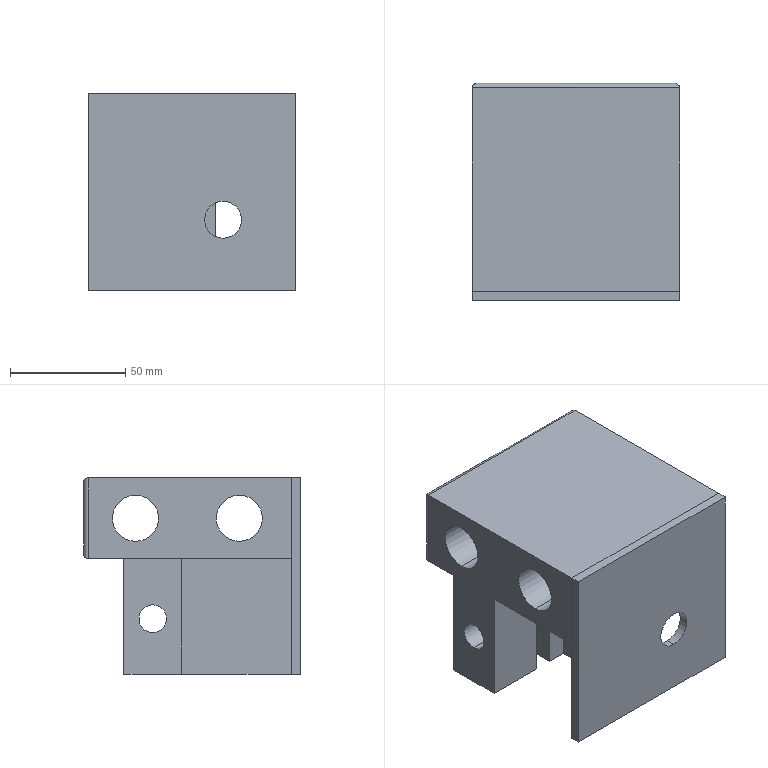Part | SolidWorks | features ICE 4, Cut 1, Extrusion 1, Fillet 1 | 4 solids | 44 faces | box 90 x 94 x 85 mm | volume 324931 mm3 | plane 28 | cylinder 16 | commonest cylinder face diameters 4 x6 12 x4 20 x4 16 x2
STEP:
#1=CARTESIAN_POINT('',(45.,22.5,-7.5));
#2=VERTEX_POINT('',#1);
#3=CARTESIAN_POINT('',(45.,22.5,-27.5));
#4=VERTEX_POINT('',#3);
#5=CARTESIAN_POINT('',(45.,22.5,-17.5));
#6=DIRECTION('',(1.,0.,0.));
#7=DIRECTION('',(0.,0.,-1.));
#8=AXIS2_PLACEMENT_3D('',#5,#6,#7);
#9=CIRCLE('',#8,10.);
#10=EDGE_CURVE('',#2,#4,#9,.T.);
#11=ORIENTED_EDGE('',*,*,#10,.T.);
#12=CARTESIAN_POINT('',(-45.,22.5,-27.5));
#13=VERTEX_POINT('',#12);
#14=CARTESIAN_POINT('',(45.,22.5,-27.5));
#15=DIRECTION('',(-1.,0.,0.));
#16=VECTOR('',#15,1000.);
#17=LINE('',#14,#16);
#18=EDGE_CURVE('',#4,#13,#17,.T.);
#19=ORIENTED_EDGE('',*,*,#18,.T.);
#20=CARTESIAN_POINT('',(-45.,22.5,-7.5));
#21=VERTEX_POINT('',#20);
#22=CARTESIAN_POINT('',(-45.,22.5,-17.5));
#23=DIRECTION('',(1.,0.,0.));
#24=DIRECTION('',(0.,0.,-1.));
#25=AXIS2_PLACEMENT_3D('',#22,#23,#24);
#26=CIRCLE('',#25,10.);
#27=EDGE_CURVE('',#21,#13,#26,.T.);
#28=ORIENTED_EDGE('',*,*,#27,.F.);
#29=CARTESIAN_POINT('',(45.,22.5,-7.5));
#30=DIRECTION('',(-1.,0.,0.));
#31=VECTOR('',#30,1000.);
#32=LINE('',#29,#31);
#33=EDGE_CURVE('',#2,#21,#32,.T.);
#34=ORIENTED_EDGE('',*,*,#33,.F.);
#35=EDGE_LOOP('',(#11,#19,#28,#34));
#36=FACE_OUTER_BOUND('',#35,.T.);
#37=CARTESIAN_POINT('',(45.,22.5,-17.5));
#38=DIRECTION('',(-1.,0.,0.));
#39=DIRECTION('',(0.,0.,1.));
#40=AXIS2_PLACEMENT_3D('',#37,#38,#39);
#41=CYLINDRICAL_SURFACE('',#40,10.);
#42=ADVANCED_FACE('',(#36),#41,.F.);
#43=CARTESIAN_POINT('',(45.,67.5,-7.5));
#44=VERTEX_POINT('',#43);
#45=CARTESIAN_POINT('',(45.,67.5,-27.5));
#46=VERTEX_POINT('',#45);
#47=CARTESIAN_POINT('',(45.,67.5,-17.5));
#48=DIRECTION('',(1.,0.,0.));
#49=DIRECTION('',(0.,0.,-1.));
#50=AXIS2_PLACEMENT_3D('',#47,#48,#49);
#51=CIRCLE('',#50,10.);
#52=EDGE_CURVE('',#44,#46,#51,.T.);
#53=ORIENTED_EDGE('',*,*,#52,.T.);
#54=CARTESIAN_POINT('',(-45.,67.5,-27.5));
#55=VERTEX_POINT('',#54);
#56=CARTESIAN_POINT('',(45.,67.5,-27.5));
#57=DIRECTION('',(-1.,0.,0.));
#58=VECTOR('',#57,1000.);
#59=LINE('',#56,#58);
#60=EDGE_CURVE('',#46,#55,#59,.T.);
#61=ORIENTED_EDGE('',*,*,#60,.T.);
#62=CARTESIAN_POINT('',(-45.,67.5,-7.5));
#63=VERTEX_POINT('',#62);
#64=CARTESIAN_POINT('',(-45.,67.5,-17.5));
#65=DIRECTION('',(1.,0.,0.));
#66=DIRECTION('',(0.,0.,-1.));
#67=AXIS2_PLACEMENT_3D('',#64,#65,#66);
#68=CIRCLE('',#67,10.);
#69=EDGE_CURVE('',#63,#55,#68,.T.);
#70=ORIENTED_EDGE('',*,*,#69,.F.);
#71=CARTESIAN_POINT('',(45.,67.5,-7.5));
#72=DIRECTION('',(-1.,0.,0.));
#73=VECTOR('',#72,1000.);
#74=LINE('',#71,#73);
#75=EDGE_CURVE('',#44,#63,#74,.T.);
#76=ORIENTED_EDGE('',*,*,#75,.F.);
#77=EDGE_LOOP('',(#53,#61,#70,#76));
#78=FACE_OUTER_BOUND('',#77,.T.);
#79=CARTESIAN_POINT('',(45.,67.5,-17.5));
#80=DIRECTION('',(-1.,0.,0.));
#81=DIRECTION('',(0.,0.,1.));
#82=AXIS2_PLACEMENT_3D('',#79,#80,#81);
#83=CYLINDRICAL_SURFACE('',#82,10.);
#84=ADVANCED_FACE('',(#78),#83,.F.);
#85=CARTESIAN_POINT('',(-45.,0.,0.));
#86=VERTEX_POINT('',#85);
#87=CARTESIAN_POINT('',(-45.,0.,-35.));
#88=VERTEX_POINT('',#87);
#89=CARTESIAN_POINT('',(-45.,0.,0.));
#90=DIRECTION('',(0.,0.,-1.));
#91=VECTOR('',#90,1000.);
#92=LINE('',#89,#91);
#93=EDGE_CURVE('',#86,#88,#92,.T.);
#94=ORIENTED_EDGE('',*,*,#93,.T.);
#95=CARTESIAN_POINT('',(45.,0.,-35.));
#96=VERTEX_POINT('',#95);
#97=CARTESIAN_POINT('',(45.,0.,-35.));
#98=DIRECTION('',(-1.,0.,0.));
#99=VECTOR('',#98,1000.);
#100=LINE('',#97,#99);
#101=EDGE_CURVE('',#96,#88,#100,.T.);
#102=ORIENTED_EDGE('',*,*,#101,.F.);
#103=CARTESIAN_POINT('',(45.,0.,0.));
#104=VERTEX_POINT('',#103);
#105=CARTESIAN_POINT('',(45.,0.,0.));
#106=DIRECTION('',(0.,0.,-1.));
#107=VECTOR('',#106,1000.);
#108=LINE('',#105,#107);
#109=EDGE_CURVE('',#104,#96,#108,.T.);
#110=ORIENTED_EDGE('',*,*,#109,.F.);
#111=CARTESIAN_POINT('',(45.,0.,0.));
#112=DIRECTION('',(-1.,0.,0.));
#113=VECTOR('',#112,1000.);
#114=LINE('',#111,#113);
#115=EDGE_CURVE('',#104,#86,#114,.T.);
#116=ORIENTED_EDGE('',*,*,#115,.T.);
#117=EDGE_LOOP('',(#94,#102,#110,#116));
#118=FACE_OUTER_BOUND('',#117,.T.);
#119=CARTESIAN_POINT('',(45.,0.,0.));
#120=DIRECTION('',(0.,1.,0.));
#121=DIRECTION('',(0.,0.,1.));
#122=AXIS2_PLACEMENT_3D('',#119,#120,#121);
#123=PLANE('',#122);
#124=ADVANCED_FACE('',(#118),#123,.F.);
#125=CARTESIAN_POINT('',(-45.,88.,-35.));
#126=VERTEX_POINT('',#125);
#127=CARTESIAN_POINT('',(-45.,0.,-35.));
#128=DIRECTION('',(0.,1.,0.));
#129=VECTOR('',#128,1000.);
#130=LINE('',#127,#129);
#131=EDGE_CURVE('',#88,#126,#130,.T.);
#132=ORIENTED_EDGE('',*,*,#131,.T.);
#133=CARTESIAN_POINT('',(45.,88.,-35.));
#134=VERTEX_POINT('',#133);
#135=CARTESIAN_POINT('',(45.,88.,-35.));
#136=DIRECTION('',(1.,0.,0.));
#137=VECTOR('',#136,1000.);
#138=LINE('',#135,#137);
#139=EDGE_CURVE('',#126,#134,#138,.T.);
#140=ORIENTED_EDGE('',*,*,#139,.T.);
#141=CARTESIAN_POINT('',(45.,0.,-35.));
#142=DIRECTION('',(0.,1.,0.));
#143=VECTOR('',#142,1000.);
#144=LINE('',#141,#143);
#145=EDGE_CURVE('',#96,#134,#144,.T.);
#146=ORIENTED_EDGE('',*,*,#145,.F.);
#147=ORIENTED_EDGE('',*,*,#101,.T.);
#148=EDGE_LOOP('',(#132,#140,#146,#147));
#149=FACE_OUTER_BOUND('',#148,.T.);
#150=CARTESIAN_POINT('',(45.,0.,-35.));
#151=DIRECTION('',(0.,0.,1.));
#152=DIRECTION('',(1.,0.,0.));
#153=AXIS2_PLACEMENT_3D('',#150,#151,#152);
#154=PLANE('',#153);
#155=ADVANCED_FACE('',(#149),#154,.F.);
#156=CARTESIAN_POINT('',(43.,90.,-2.));
#157=VERTEX_POINT('',#156);
#158=CARTESIAN_POINT('',(43.,90.,-33.));
#159=VERTEX_POINT('',#158);
#160=CARTESIAN_POINT('',(43.,90.,0.));
#161=DIRECTION('',(0.,0.,-1.));
#162=VECTOR('',#161,1000.);
#163=LINE('',#160,#162);
#164=EDGE_CURVE('',#157,#159,#163,.T.);
#165=ORIENTED_EDGE('',*,*,#164,.T.);
#166=CARTESIAN_POINT('',(-43.,90.,-33.));
#167=VERTEX_POINT('',#166);
#168=CARTESIAN_POINT('',(-45.,90.,-33.));
#169=DIRECTION('',(-1.,0.,0.));
#170=VECTOR('',#169,1000.);
#171=LINE('',#168,#170);
#172=EDGE_CURVE('',#159,#167,#171,.T.);
#173=ORIENTED_EDGE('',*,*,#172,.T.);
#174=CARTESIAN_POINT('',(-43.,90.,-2.));
#175=VERTEX_POINT('',#174);
#176=CARTESIAN_POINT('',(-43.,90.,0.));
#177=DIRECTION('',(0.,0.,1.));
#178=VECTOR('',#177,1000.);
#179=LINE('',#176,#178);
#180=EDGE_CURVE('',#167,#175,#179,.T.);
#181=ORIENTED_EDGE('',*,*,#180,.T.);
#182=CARTESIAN_POINT('',(45.,90.,-2.));
#183=DIRECTION('',(1.,0.,0.));
#184=VECTOR('',#183,1000.);
#185=LINE('',#182,#184);
#186=EDGE_CURVE('',#175,#157,#185,.T.);
#187=ORIENTED_EDGE('',*,*,#186,.T.);
#188=EDGE_LOOP('',(#165,#173,#181,#187));
#189=FACE_OUTER_BOUND('',#188,.T.);
#190=CARTESIAN_POINT('',(45.,90.,0.));
#191=DIRECTION('',(0.,1.,0.));
#192=DIRECTION('',(0.,0.,1.));
#193=AXIS2_PLACEMENT_3D('',#190,#191,#192);
#194=PLANE('',#193);
#195=ADVANCED_FACE('',(#189),#194,.T.);
#196=ORIENTED_EDGE('',*,*,#60,.F.);
#197=CARTESIAN_POINT('',(45.,67.5,-17.5));
#198=DIRECTION('',(1.,0.,0.));
#199=DIRECTION('',(0.,0.,-1.));
#200=AXIS2_PLACEMENT_3D('',#197,#198,#199);
#201=CIRCLE('',#200,10.);
#202=EDGE_CURVE('',#46,#44,#201,.T.);
#203=ORIENTED_EDGE('',*,*,#202,.T.);
#204=ORIENTED_EDGE('',*,*,#75,.T.);
#205=CARTESIAN_POINT('',(-45.,67.5,-17.5));
#206=DIRECTION('',(1.,0.,0.));
#207=DIRECTION('',(0.,0.,-1.));
#208=AXIS2_PLACEMENT_3D('',#205,#206,#207);
#209=CIRCLE('',#208,10.);
#210=EDGE_CURVE('',#55,#63,#209,.T.);
#211=ORIENTED_EDGE('',*,*,#210,.F.);
#212=EDGE_LOOP('',(#196,#203,#204,#211));
#213=FACE_OUTER_BOUND('',#212,.T.);
#214=CARTESIAN_POINT('',(45.,67.5,-17.5));
#215=DIRECTION('',(-1.,0.,0.));
#216=DIRECTION('',(0.,0.,1.));
#217=AXIS2_PLACEMENT_3D('',#214,#215,#216);
#218=CYLINDRICAL_SURFACE('',#217,10.);
#219=ADVANCED_FACE('',(#213),#218,.F.);
#220=ORIENTED_EDGE('',*,*,#18,.F.);
#221=CARTESIAN_POINT('',(45.,22.5,-17.5));
#222=DIRECTION('',(1.,0.,0.));
#223=DIRECTION('',(0.,0.,-1.));
#224=AXIS2_PLACEMENT_3D('',#221,#222,#223);
#225=CIRCLE('',#224,10.);
#226=EDGE_CURVE('',#4,#2,#225,.T.);
#227=ORIENTED_EDGE('',*,*,#226,.T.);
#228=ORIENTED_EDGE('',*,*,#33,.T.);
#229=CARTESIAN_POINT('',(-45.,22.5,-17.5));
#230=DIRECTION('',(1.,0.,0.));
#231=DIRECTION('',(0.,0.,-1.));
#232=AXIS2_PLACEMENT_3D('',#229,#230,#231);
#233=CIRCLE('',#232,10.);
#234=EDGE_CURVE('',#13,#21,#233,.T.);
#235=ORIENTED_EDGE('',*,*,#234,.F.);
#236=EDGE_LOOP('',(#220,#227,#228,#235));
#237=FACE_OUTER_BOUND('',#236,.T.);
#238=CARTESIAN_POINT('',(45.,22.5,-17.5));
#239=DIRECTION('',(-1.,0.,0.));
#240=DIRECTION('',(0.,0.,1.));
#241=AXIS2_PLACEMENT_3D('',#238,#239,#240);
#242=CYLINDRICAL_SURFACE('',#241,10.);
#243=ADVANCED_FACE('',(#237),#242,.F.);
#244=CARTESIAN_POINT('',(45.,88.,0.));
#245=VERTEX_POINT('',#244);
#246=CARTESIAN_POINT('',(45.,0.,0.));
#247=DIRECTION('',(0.,1.,0.));
#248=VECTOR('',#247,1000.);
#249=LINE('',#246,#248);
#250=EDGE_CURVE('',#104,#245,#249,.T.);
#251=ORIENTED_EDGE('',*,*,#250,.T.);
#252=CARTESIAN_POINT('',(-45.,88.,0.));
#253=VERTEX_POINT('',#252);
#254=CARTESIAN_POINT('',(45.,88.,0.));
#255=DIRECTION('',(-1.,0.,0.));
#256=VECTOR('',#255,1000.);
#257=LINE('',#254,#256);
#258=EDGE_CURVE('',#245,#253,#257,.T.);
#259=ORIENTED_EDGE('',*,*,#258,.T.);
#260=CARTESIAN_POINT('',(-45.,0.,0.));
#261=DIRECTION('',(0.,1.,0.));
#262=VECTOR('',#261,1000.);
#263=LINE('',#260,#262);
#264=EDGE_CURVE('',#86,#253,#263,.T.);
#265=ORIENTED_EDGE('',*,*,#264,.F.);
#266=ORIENTED_EDGE('',*,*,#115,.F.);
#267=EDGE_LOOP('',(#251,#259,#265,#266));
#268=FACE_OUTER_BOUND('',#267,.T.);
#269=CARTESIAN_POINT('',(45.,0.,0.));
#270=DIRECTION('',(0.,0.,1.));
#271=DIRECTION('',(1.,0.,0.));
#272=AXIS2_PLACEMENT_3D('',#269,#270,#271);
#273=PLANE('',#272);
#274=ADVANCED_FACE('',(#268),#273,.T.);
#275=ORIENTED_EDGE('',*,*,#10,.F.);
#276=ORIENTED_EDGE('',*,*,#226,.F.);
#277=EDGE_LOOP('',(#275,#276));
#278=FACE_BOUND('',#277,.T.);
#279=ORIENTED_EDGE('',*,*,#52,.F.);
#280=ORIENTED_EDGE('',*,*,#202,.F.);
#281=EDGE_LOOP('',(#279,#280));
#282=FACE_BOUND('',#281,.T.);
#283=ORIENTED_EDGE('',*,*,#145,.T.);
#284=CARTESIAN_POINT('',(45.,88.,0.));
#285=DIRECTION('',(0.,0.,1.));
#286=VECTOR('',#285,1000.);
#287=LINE('',#284,#286);
#288=EDGE_CURVE('',#134,#245,#287,.T.);
#289=ORIENTED_EDGE('',*,*,#288,.T.);
#290=ORIENTED_EDGE('',*,*,#250,.F.);
#291=ORIENTED_EDGE('',*,*,#109,.T.);
#292=EDGE_LOOP('',(#283,#289,#290,#291));
#293=FACE_OUTER_BOUND('',#292,.T.);
#294=CARTESIAN_POINT('',(45.,0.,0.));
#295=DIRECTION('',(1.,0.,0.));
#296=DIRECTION('',(0.,0.,-1.));
#297=AXIS2_PLACEMENT_3D('',#294,#295,#296);
#298=PLANE('',#297);
#299=ADVANCED_FACE('',(#278,#282,#293),#298,.T.);
#300=ORIENTED_EDGE('',*,*,#27,.T.);
#301=ORIENTED_EDGE('',*,*,#234,.T.);
#302=EDGE_LOOP('',(#300,#301));
#303=FACE_BOUND('',#302,.T.);
#304=ORIENTED_EDGE('',*,*,#69,.T.);
#305=ORIENTED_EDGE('',*,*,#210,.T.);
#306=EDGE_LOOP('',(#304,#305));
#307=FACE_BOUND('',#306,.T.);
#308=ORIENTED_EDGE('',*,*,#264,.T.);
#309=CARTESIAN_POINT('',(-45.,88.,-35.));
#310=DIRECTION('',(0.,0.,-1.));
#311=VECTOR('',#310,1000.);
#312=LINE('',#309,#311);
#313=EDGE_CURVE('',#253,#126,#312,.T.);
#314=ORIENTED_EDGE('',*,*,#313,.T.);
#315=ORIENTED_EDGE('',*,*,#131,.F.);
#316=ORIENTED_EDGE('',*,*,#93,.F.);
#317=EDGE_LOOP('',(#308,#314,#315,#316));
#318=FACE_OUTER_BOUND('',#317,.T.);
#319=CARTESIAN_POINT('',(-45.,0.,0.));
#320=DIRECTION('',(1.,0.,0.));
#321=DIRECTION('',(0.,0.,-1.));
#322=AXIS2_PLACEMENT_3D('',#319,#320,#321);
#323=PLANE('',#322);
#324=ADVANCED_FACE('',(#303,#307,#318),#323,.F.);
#325=CARTESIAN_POINT('',(-45.,88.,0.));
#326=CARTESIAN_POINT('',(-45.,89.172,0.));
#327=CARTESIAN_POINT('',(-44.172,90.,-0.8284));
#328=CARTESIAN_POINT('',(-43.,90.,-2.));
#329=(BOUNDED_CURVE()B_SPLINE_CURVE(3,(#325,#326,#327,#328),.UNSPECIFIED.,.F.,.F.)B_SPLINE_CURVE_WITH_KNOTS((4,4),(0.,1.571),.UNSPECIFIED.)CURVE()GEOMETRIC_REPRESENTATION_ITEM()RATIONAL_B_SPLINE_CURVE((1.,0.8047,0.8047,1.))REPRESENTATION_ITEM(''));
#330=EDGE_CURVE('',#253,#175,#329,.T.);
#331=ORIENTED_EDGE('',*,*,#330,.F.);
#332=ORIENTED_EDGE('',*,*,#258,.F.);
#333=CARTESIAN_POINT('',(43.,90.,-2.));
#334=CARTESIAN_POINT('',(44.172,90.,-0.8284));
#335=CARTESIAN_POINT('',(45.,89.172,0.));
#336=CARTESIAN_POINT('',(45.,88.,0.));
#337=(BOUNDED_CURVE()B_SPLINE_CURVE(3,(#333,#334,#335,#336),.UNSPECIFIED.,.F.,.F.)B_SPLINE_CURVE_WITH_KNOTS((4,4),(1.571,3.142),.UNSPECIFIED.)CURVE()GEOMETRIC_REPRESENTATION_ITEM()RATIONAL_B_SPLINE_CURVE((1.,0.8047,0.8047,1.))REPRESENTATION_ITEM(''));
#338=EDGE_CURVE('',#157,#245,#337,.T.);
#339=ORIENTED_EDGE('',*,*,#338,.F.);
#340=ORIENTED_EDGE('',*,*,#186,.F.);
#341=EDGE_LOOP('',(#331,#332,#339,#340));
#342=FACE_OUTER_BOUND('',#341,.T.);
#343=CARTESIAN_POINT('',(45.,88.,-2.));
#344=DIRECTION('',(-1.,0.,0.));
#345=DIRECTION('',(0.,0.,1.));
#346=AXIS2_PLACEMENT_3D('',#343,#344,#345);
#347=CYLINDRICAL_SURFACE('',#346,2.);
#348=ADVANCED_FACE('',(#342),#347,.T.);
#349=ORIENTED_EDGE('',*,*,#338,.T.);
#350=ORIENTED_EDGE('',*,*,#288,.F.);
#351=CARTESIAN_POINT('',(43.,90.,-33.));
#352=CARTESIAN_POINT('',(44.172,90.,-34.172));
#353=CARTESIAN_POINT('',(45.,89.172,-35.));
#354=CARTESIAN_POINT('',(45.,88.,-35.));
#355=(BOUNDED_CURVE()B_SPLINE_CURVE(3,(#351,#352,#353,#354),.UNSPECIFIED.,.F.,.T.)B_SPLINE_CURVE_WITH_KNOTS((4,4),(4.712,6.283),.UNSPECIFIED.)CURVE()GEOMETRIC_REPRESENTATION_ITEM()RATIONAL_B_SPLINE_CURVE((1.,0.8047,0.8047,1.))REPRESENTATION_ITEM(''));
#356=EDGE_CURVE('',#159,#134,#355,.T.);
#357=ORIENTED_EDGE('',*,*,#356,.F.);
#358=ORIENTED_EDGE('',*,*,#164,.F.);
#359=EDGE_LOOP('',(#349,#350,#357,#358));
#360=FACE_OUTER_BOUND('',#359,.T.);
#361=CARTESIAN_POINT('',(43.,88.,0.));
#362=DIRECTION('',(0.,0.,-1.));
#363=DIRECTION('',(-1.,0.,0.));
#364=AXIS2_PLACEMENT_3D('',#361,#362,#363);
#365=CYLINDRICAL_SURFACE('',#364,2.);
#366=ADVANCED_FACE('',(#360),#365,.T.);
#367=ORIENTED_EDGE('',*,*,#330,.T.);
#368=ORIENTED_EDGE('',*,*,#180,.F.);
#369=CARTESIAN_POINT('',(-45.,88.,-35.));
#370=CARTESIAN_POINT('',(-45.,89.172,-35.));
#371=CARTESIAN_POINT('',(-44.172,90.,-34.172));
#372=CARTESIAN_POINT('',(-43.,90.,-33.));
#373=(BOUNDED_CURVE()B_SPLINE_CURVE(3,(#369,#370,#371,#372),.UNSPECIFIED.,.F.,.F.)B_SPLINE_CURVE_WITH_KNOTS((4,4),(3.142,4.712),.UNSPECIFIED.)CURVE()GEOMETRIC_REPRESENTATION_ITEM()RATIONAL_B_SPLINE_CURVE((1.,0.8047,0.8047,1.))REPRESENTATION_ITEM(''));
#374=EDGE_CURVE('',#126,#167,#373,.T.);
#375=ORIENTED_EDGE('',*,*,#374,.F.);
#376=ORIENTED_EDGE('',*,*,#313,.F.);
#377=EDGE_LOOP('',(#367,#368,#375,#376));
#378=FACE_OUTER_BOUND('',#377,.T.);
#379=CARTESIAN_POINT('',(-43.,88.,0.));
#380=DIRECTION('',(0.,0.,1.));
#381=DIRECTION('',(1.,0.,0.));
#382=AXIS2_PLACEMENT_3D('',#379,#380,#381);
#383=CYLINDRICAL_SURFACE('',#382,2.);
#384=ADVANCED_FACE('',(#378),#383,.T.);
#385=ORIENTED_EDGE('',*,*,#356,.T.);
#386=ORIENTED_EDGE('',*,*,#139,.F.);
#387=ORIENTED_EDGE('',*,*,#374,.T.);
#388=ORIENTED_EDGE('',*,*,#172,.F.);
#389=EDGE_LOOP('',(#385,#386,#387,#388));
#390=FACE_OUTER_BOUND('',#389,.T.);
#391=CARTESIAN_POINT('',(45.,88.,-33.));
#392=DIRECTION('',(1.,0.,0.));
#393=DIRECTION('',(0.,0.,-1.));
#394=AXIS2_PLACEMENT_3D('',#391,#392,#393);
#395=CYLINDRICAL_SURFACE('',#394,2.);
#396=ADVANCED_FACE('',(#390),#395,.T.);
#397=CLOSED_SHELL('',(#42,#84,#124,#155,#195,#219,#243,#274,#299,#324,#348,#366,#384,#396));
#398=MANIFOLD_SOLID_BREP('',#397);
#399=CARTESIAN_POINT('',(10.,60.,-55.));
#400=VERTEX_POINT('',#399);
#401=CARTESIAN_POINT('',(10.,60.,-67.));
#402=VERTEX_POINT('',#401);
#403=CARTESIAN_POINT('',(10.,60.,-61.));
#404=DIRECTION('',(1.,0.,0.));
#405=DIRECTION('',(0.,0.,1.));
#406=AXIS2_PLACEMENT_3D('',#403,#404,#405);
#407=CIRCLE('',#406,6.);
#408=EDGE_CURVE('',#400,#402,#407,.T.);
#409=ORIENTED_EDGE('',*,*,#408,.T.);
#410=CARTESIAN_POINT('',(-11.,60.,-67.));
#411=VERTEX_POINT('',#410);
#412=CARTESIAN_POINT('',(45.,60.,-67.));
#413=DIRECTION('',(-1.,0.,0.));
#414=VECTOR('',#413,1000.);
#415=LINE('',#412,#414);
#416=EDGE_CURVE('',#402,#411,#415,.T.);
#417=ORIENTED_EDGE('',*,*,#416,.T.);
#418=CARTESIAN_POINT('',(-11.,60.,-55.));
#419=VERTEX_POINT('',#418);
#420=CARTESIAN_POINT('',(-11.,60.,-61.));
#421=DIRECTION('',(-1.,0.,0.));
#422=DIRECTION('',(0.,0.,-1.));
#423=AXIS2_PLACEMENT_3D('',#420,#421,#422);
#424=CIRCLE('',#423,6.);
#425=EDGE_CURVE('',#411,#419,#424,.T.);
#426=ORIENTED_EDGE('',*,*,#425,.T.);
#427=CARTESIAN_POINT('',(45.,60.,-55.));
#428=DIRECTION('',(-1.,0.,0.));
#429=VECTOR('',#428,1000.);
#430=LINE('',#427,#429);
#431=EDGE_CURVE('',#400,#419,#430,.T.);
#432=ORIENTED_EDGE('',*,*,#431,.F.);
#433=EDGE_LOOP('',(#409,#417,#426,#432));
#434=FACE_OUTER_BOUND('',#433,.T.);
#435=CARTESIAN_POINT('',(45.,60.,-61.));
#436=DIRECTION('',(-1.,0.,0.));
#437=DIRECTION('',(0.,0.,1.));
#438=AXIS2_PLACEMENT_3D('',#435,#436,#437);
#439=CYLINDRICAL_SURFACE('',#438,6.);
#440=ADVANCED_FACE('',(#434),#439,.F.);
#441=CARTESIAN_POINT('',(-15.,47.5,-45.));
#442=VERTEX_POINT('',#441);
#443=CARTESIAN_POINT('',(-15.,47.5,-49.));
#444=VERTEX_POINT('',#443);
#445=CARTESIAN_POINT('',(-15.,47.5,-47.));
#446=DIRECTION('',(0.,-1.,0.));
#447=DIRECTION('',(0.,0.,1.));
#448=AXIS2_PLACEMENT_3D('',#445,#446,#447);
#449=CIRCLE('',#448,2.);
#450=EDGE_CURVE('',#442,#444,#449,.T.);
#451=ORIENTED_EDGE('',*,*,#450,.T.);
#452=CARTESIAN_POINT('',(-15.,72.5,-49.));
#453=VERTEX_POINT('',#452);
#454=CARTESIAN_POINT('',(-15.,-4.001,-49.));
#455=DIRECTION('',(0.,1.,0.));
#456=VECTOR('',#455,1000.);
#457=LINE('',#454,#456);
#458=EDGE_CURVE('',#444,#453,#457,.T.);
#459=ORIENTED_EDGE('',*,*,#458,.T.);
#460=CARTESIAN_POINT('',(-15.,72.5,-45.));
#461=VERTEX_POINT('',#460);
#462=CARTESIAN_POINT('',(-15.,72.5,-47.));
#463=DIRECTION('',(0.,1.,0.));
#464=DIRECTION('',(0.,0.,1.));
#465=AXIS2_PLACEMENT_3D('',#462,#463,#464);
#466=CIRCLE('',#465,2.);
#467=EDGE_CURVE('',#453,#461,#466,.T.);
#468=ORIENTED_EDGE('',*,*,#467,.T.);
#469=CARTESIAN_POINT('',(-15.,-4.001,-45.));
#470=DIRECTION('',(0.,1.,0.));
#471=VECTOR('',#470,1000.);
#472=LINE('',#469,#471);
#473=EDGE_CURVE('',#442,#461,#472,.T.);
#474=ORIENTED_EDGE('',*,*,#473,.F.);
#475=EDGE_LOOP('',(#451,#459,#468,#474));
#476=FACE_OUTER_BOUND('',#475,.T.);
#477=CARTESIAN_POINT('',(-15.,-4.001,-47.));
#478=DIRECTION('',(0.,1.,0.));
#479=DIRECTION('',(0.,0.,1.));
#480=AXIS2_PLACEMENT_3D('',#477,#478,#479);
#481=CYLINDRICAL_SURFACE('',#480,2.);
#482=ADVANCED_FACE('',(#476),#481,.F.);
#483=CARTESIAN_POINT('',(-19.,60.,-55.));
#484=VERTEX_POINT('',#483);
#485=CARTESIAN_POINT('',(-19.,60.,-67.));
#486=VERTEX_POINT('',#485);
#487=CARTESIAN_POINT('',(-19.,60.,-61.));
#488=DIRECTION('',(1.,0.,0.));
#489=DIRECTION('',(0.,0.,1.));
#490=AXIS2_PLACEMENT_3D('',#487,#488,#489);
#491=CIRCLE('',#490,6.);
#492=EDGE_CURVE('',#484,#486,#491,.T.);
#493=ORIENTED_EDGE('',*,*,#492,.T.);
#494=CARTESIAN_POINT('',(-45.,60.,-67.));
#495=VERTEX_POINT('',#494);
#496=CARTESIAN_POINT('',(45.,60.,-67.));
#497=DIRECTION('',(-1.,0.,0.));
#498=VECTOR('',#497,1000.);
#499=LINE('',#496,#498);
#500=EDGE_CURVE('',#486,#495,#499,.T.);
#501=ORIENTED_EDGE('',*,*,#500,.T.);
#502=CARTESIAN_POINT('',(-45.,60.,-55.));
#503=VERTEX_POINT('',#502);
#504=CARTESIAN_POINT('',(-45.,60.,-61.));
#505=DIRECTION('',(1.,0.,0.));
#506=DIRECTION('',(0.,0.,-1.));
#507=AXIS2_PLACEMENT_3D('',#504,#505,#506);
#508=CIRCLE('',#507,6.);
#509=EDGE_CURVE('',#503,#495,#508,.T.);
#510=ORIENTED_EDGE('',*,*,#509,.F.);
#511=CARTESIAN_POINT('',(45.,60.,-55.));
#512=DIRECTION('',(-1.,0.,0.));
#513=VECTOR('',#512,1000.);
#514=LINE('',#511,#513);
#515=EDGE_CURVE('',#484,#503,#514,.T.);
#516=ORIENTED_EDGE('',*,*,#515,.F.);
#517=EDGE_LOOP('',(#493,#501,#510,#516));
#518=FACE_OUTER_BOUND('',#517,.T.);
#519=CARTESIAN_POINT('',(45.,60.,-61.));
#520=DIRECTION('',(-1.,0.,0.));
#521=DIRECTION('',(0.,0.,1.));
#522=AXIS2_PLACEMENT_3D('',#519,#520,#521);
#523=CYLINDRICAL_SURFACE('',#522,6.);
#524=ADVANCED_FACE('',(#518),#523,.F.);
#525=ORIENTED_EDGE('',*,*,#500,.F.);
#526=CARTESIAN_POINT('',(-19.,60.,-61.));
#527=DIRECTION('',(1.,0.,0.));
#528=DIRECTION('',(0.,0.,1.));
#529=AXIS2_PLACEMENT_3D('',#526,#527,#528);
#530=CIRCLE('',#529,6.);
#531=EDGE_CURVE('',#486,#484,#530,.T.);
#532=ORIENTED_EDGE('',*,*,#531,.T.);
#533=ORIENTED_EDGE('',*,*,#515,.T.);
#534=CARTESIAN_POINT('',(-45.,60.,-61.));
#535=DIRECTION('',(1.,0.,0.));
#536=DIRECTION('',(0.,0.,-1.));
#537=AXIS2_PLACEMENT_3D('',#534,#535,#536);
#538=CIRCLE('',#537,6.);
#539=EDGE_CURVE('',#495,#503,#538,.T.);
#540=ORIENTED_EDGE('',*,*,#539,.F.);
#541=EDGE_LOOP('',(#525,#532,#533,#540));
#542=FACE_OUTER_BOUND('',#541,.T.);
#543=CARTESIAN_POINT('',(45.,60.,-61.));
#544=DIRECTION('',(-1.,0.,0.));
#545=DIRECTION('',(0.,0.,1.));
#546=AXIS2_PLACEMENT_3D('',#543,#544,#545);
#547=CYLINDRICAL_SURFACE('',#546,6.);
#548=ADVANCED_FACE('',(#542),#547,.F.);
#549=ORIENTED_EDGE('',*,*,#509,.T.);
#550=ORIENTED_EDGE('',*,*,#539,.T.);
#551=EDGE_LOOP('',(#549,#550));
#552=FACE_BOUND('',#551,.T.);
#553=CARTESIAN_POINT('',(-45.,72.5,-85.));
#554=VERTEX_POINT('',#553);
#555=CARTESIAN_POINT('',(-45.,47.5,-85.));
#556=VERTEX_POINT('',#555);
#557=CARTESIAN_POINT('',(-45.,0.,-85.));
#558=DIRECTION('',(0.,-1.,0.));
#559=VECTOR('',#558,1000.);
#560=LINE('',#557,#559);
#561=EDGE_CURVE('',#554,#556,#560,.T.);
#562=ORIENTED_EDGE('',*,*,#561,.T.);
#563=CARTESIAN_POINT('',(-45.,47.5,-35.));
#564=VERTEX_POINT('',#563);
#565=CARTESIAN_POINT('',(-45.,47.5,0.));
#566=DIRECTION('',(0.,0.,-1.));
#567=VECTOR('',#566,1000.);
#568=LINE('',#565,#567);
#569=EDGE_CURVE('',#564,#556,#568,.T.);
#570=ORIENTED_EDGE('',*,*,#569,.F.);
#571=CARTESIAN_POINT('',(-45.,72.5,-35.));
#572=VERTEX_POINT('',#571);
#573=CARTESIAN_POINT('',(-45.,0.,-35.));
#574=DIRECTION('',(0.,1.,0.));
#575=VECTOR('',#574,1000.);
#576=LINE('',#573,#575);
#577=EDGE_CURVE('',#564,#572,#576,.T.);
#578=ORIENTED_EDGE('',*,*,#577,.T.);
#579=CARTESIAN_POINT('',(-45.,72.5,0.));
#580=DIRECTION('',(0.,0.,1.));
#581=VECTOR('',#580,1000.);
#582=LINE('',#579,#581);
#583=EDGE_CURVE('',#554,#572,#582,.T.);
#584=ORIENTED_EDGE('',*,*,#583,.F.);
#585=EDGE_LOOP('',(#562,#570,#578,#584));
#586=FACE_OUTER_BOUND('',#585,.T.);
#587=CARTESIAN_POINT('',(-45.,0.,0.));
#588=DIRECTION('',(1.,0.,0.));
#589=DIRECTION('',(0.,0.,-1.));
#590=AXIS2_PLACEMENT_3D('',#587,#588,#589);
#591=PLANE('',#590);
#592=ADVANCED_FACE('',(#552,#586),#591,.F.);
#593=ORIENTED_EDGE('',*,*,#450,.F.);
#594=CARTESIAN_POINT('',(-15.,47.5,-47.));
#595=DIRECTION('',(0.,-1.,0.));
#596=DIRECTION('',(0.,0.,1.));
#597=AXIS2_PLACEMENT_3D('',#594,#595,#596);
#598=CIRCLE('',#597,2.);
#599=EDGE_CURVE('',#444,#442,#598,.T.);
#600=ORIENTED_EDGE('',*,*,#599,.F.);
#601=EDGE_LOOP('',(#593,#600));
#602=FACE_BOUND('',#601,.T.);
#603=CARTESIAN_POINT('',(10.,47.5,-85.));
#604=VERTEX_POINT('',#603);
#605=CARTESIAN_POINT('',(-11.,47.5,-85.));
#606=VERTEX_POINT('',#605);
#607=CARTESIAN_POINT('',(45.,47.5,-85.));
#608=DIRECTION('',(-1.,0.,0.));
#609=VECTOR('',#608,1000.);
#610=LINE('',#607,#609);
#611=EDGE_CURVE('',#604,#606,#610,.T.);
#612=ORIENTED_EDGE('',*,*,#611,.F.);
#613=CARTESIAN_POINT('',(10.,47.5,-35.));
#614=VERTEX_POINT('',#613);
#615=CARTESIAN_POINT('',(10.,47.5,-35.));
#616=DIRECTION('',(0.,0.,-1.));
#617=VECTOR('',#616,1000.);
#618=LINE('',#615,#617);
#619=EDGE_CURVE('',#614,#604,#618,.T.);
#620=ORIENTED_EDGE('',*,*,#619,.F.);
#621=CARTESIAN_POINT('',(45.,47.5,-35.));
#622=DIRECTION('',(-1.,0.,0.));
#623=VECTOR('',#622,1000.);
#624=LINE('',#621,#623);
#625=EDGE_CURVE('',#614,#564,#624,.T.);
#626=ORIENTED_EDGE('',*,*,#625,.T.);
#627=ORIENTED_EDGE('',*,*,#569,.T.);
#628=CARTESIAN_POINT('',(-19.,47.5,-85.));
#629=VERTEX_POINT('',#628);
#630=CARTESIAN_POINT('',(45.,47.5,-85.));
#631=DIRECTION('',(-1.,0.,0.));
#632=VECTOR('',#631,1000.);
#633=LINE('',#630,#632);
#634=EDGE_CURVE('',#629,#556,#633,.T.);
#635=ORIENTED_EDGE('',*,*,#634,.F.);
#636=CARTESIAN_POINT('',(-19.,47.5,-52.));
#637=VERTEX_POINT('',#636);
#638=CARTESIAN_POINT('',(-19.,47.5,-85.));
#639=DIRECTION('',(0.,0.,-1.));
#640=VECTOR('',#639,1000.);
#641=LINE('',#638,#640);
#642=EDGE_CURVE('',#637,#629,#641,.T.);
#643=ORIENTED_EDGE('',*,*,#642,.F.);
#644=CARTESIAN_POINT('',(-11.,47.5,-52.));
#645=VERTEX_POINT('',#644);
#646=CARTESIAN_POINT('',(-11.,47.5,-52.));
#647=DIRECTION('',(-1.,0.,0.));
#648=VECTOR('',#647,1000.);
#649=LINE('',#646,#648);
#650=EDGE_CURVE('',#645,#637,#649,.T.);
#651=ORIENTED_EDGE('',*,*,#650,.F.);
#652=CARTESIAN_POINT('',(-11.,47.5,-85.));
#653=DIRECTION('',(0.,0.,1.));
#654=VECTOR('',#653,1000.);
#655=LINE('',#652,#654);
#656=EDGE_CURVE('',#606,#645,#655,.T.);
#657=ORIENTED_EDGE('',*,*,#656,.F.);
#658=EDGE_LOOP('',(#612,#620,#626,#627,#635,#643,#651,#657));
#659=FACE_OUTER_BOUND('',#658,.T.);
#660=CARTESIAN_POINT('',(45.,47.5,0.));
#661=DIRECTION('',(0.,1.,0.));
#662=DIRECTION('',(0.,0.,1.));
#663=AXIS2_PLACEMENT_3D('',#660,#661,#662);
#664=PLANE('',#663);
#665=ADVANCED_FACE('',(#602,#659),#664,.F.);
#666=CARTESIAN_POINT('',(10.,72.5,-35.));
#667=VERTEX_POINT('',#666);
#668=CARTESIAN_POINT('',(10.,-4.001,-35.));
#669=DIRECTION('',(0.,1.,0.));
#670=VECTOR('',#669,1000.);
#671=LINE('',#668,#670);
#672=EDGE_CURVE('',#614,#667,#671,.T.);
#673=ORIENTED_EDGE('',*,*,#672,.T.);
#674=CARTESIAN_POINT('',(45.,72.5,-35.));
#675=DIRECTION('',(-1.,0.,0.));
#676=VECTOR('',#675,1000.);
#677=LINE('',#674,#676);
#678=EDGE_CURVE('',#667,#572,#677,.T.);
#679=ORIENTED_EDGE('',*,*,#678,.T.);
#680=ORIENTED_EDGE('',*,*,#577,.F.);
#681=ORIENTED_EDGE('',*,*,#625,.F.);
#682=EDGE_LOOP('',(#673,#679,#680,#681));
#683=FACE_OUTER_BOUND('',#682,.T.);
#684=CARTESIAN_POINT('',(45.,0.,-35.));
#685=DIRECTION('',(0.,0.,1.));
#686=DIRECTION('',(1.,0.,0.));
#687=AXIS2_PLACEMENT_3D('',#684,#685,#686);
#688=PLANE('',#687);
#689=ADVANCED_FACE('',(#683),#688,.T.);
#690=CARTESIAN_POINT('',(-15.,72.5,-47.));
#691=DIRECTION('',(0.,1.,0.));
#692=DIRECTION('',(0.,0.,1.));
#693=AXIS2_PLACEMENT_3D('',#690,#691,#692);
#694=CIRCLE('',#693,2.);
#695=EDGE_CURVE('',#461,#453,#694,.T.);
#696=ORIENTED_EDGE('',*,*,#695,.F.);
#697=ORIENTED_EDGE('',*,*,#467,.F.);
#698=EDGE_LOOP('',(#696,#697));
#699=FACE_BOUND('',#698,.T.);
#700=ORIENTED_EDGE('',*,*,#678,.F.);
#701=CARTESIAN_POINT('',(10.,72.5,-85.));
#702=VERTEX_POINT('',#701);
#703=CARTESIAN_POINT('',(10.,72.5,-35.));
#704=DIRECTION('',(0.,0.,1.));
#705=VECTOR('',#704,1000.);
#706=LINE('',#703,#705);
#707=EDGE_CURVE('',#702,#667,#706,.T.);
#708=ORIENTED_EDGE('',*,*,#707,.F.);
#709=CARTESIAN_POINT('',(-11.,72.5,-85.));
#710=VERTEX_POINT('',#709);
#711=CARTESIAN_POINT('',(45.,72.5,-85.));
#712=DIRECTION('',(-1.,0.,0.));
#713=VECTOR('',#712,1000.);
#714=LINE('',#711,#713);
#715=EDGE_CURVE('',#702,#710,#714,.T.);
#716=ORIENTED_EDGE('',*,*,#715,.T.);
#717=CARTESIAN_POINT('',(-11.,72.5,-52.));
#718=VERTEX_POINT('',#717);
#719=CARTESIAN_POINT('',(-11.,72.5,-85.));
#720=DIRECTION('',(0.,0.,-1.));
#721=VECTOR('',#720,1000.);
#722=LINE('',#719,#721);
#723=EDGE_CURVE('',#718,#710,#722,.T.);
#724=ORIENTED_EDGE('',*,*,#723,.F.);
#725=CARTESIAN_POINT('',(-19.,72.5,-52.));
#726=VERTEX_POINT('',#725);
#727=CARTESIAN_POINT('',(-11.,72.5,-52.));
#728=DIRECTION('',(1.,0.,0.));
#729=VECTOR('',#728,1000.);
#730=LINE('',#727,#729);
#731=EDGE_CURVE('',#726,#718,#730,.T.);
#732=ORIENTED_EDGE('',*,*,#731,.F.);
#733=CARTESIAN_POINT('',(-19.,72.5,-85.));
#734=VERTEX_POINT('',#733);
#735=CARTESIAN_POINT('',(-19.,72.5,-85.));
#736=DIRECTION('',(0.,0.,1.));
#737=VECTOR('',#736,1000.);
#738=LINE('',#735,#737);
#739=EDGE_CURVE('',#734,#726,#738,.T.);
#740=ORIENTED_EDGE('',*,*,#739,.F.);
#741=CARTESIAN_POINT('',(45.,72.5,-85.));
#742=DIRECTION('',(-1.,0.,0.));
#743=VECTOR('',#742,1000.);
#744=LINE('',#741,#743);
#745=EDGE_CURVE('',#734,#554,#744,.T.);
#746=ORIENTED_EDGE('',*,*,#745,.T.);
#747=ORIENTED_EDGE('',*,*,#583,.T.);
#748=EDGE_LOOP('',(#700,#708,#716,#724,#732,#740,#746,#747));
#749=FACE_OUTER_BOUND('',#748,.T.);
#750=CARTESIAN_POINT('',(45.,72.5,0.));
#751=DIRECTION('',(0.,-1.,0.));
#752=DIRECTION('',(0.,0.,-1.));
#753=AXIS2_PLACEMENT_3D('',#750,#751,#752);
#754=PLANE('',#753);
#755=ADVANCED_FACE('',(#699,#749),#754,.F.);
#756=CARTESIAN_POINT('',(-19.,-4.001,-85.));
#757=DIRECTION('',(0.,1.,0.));
#758=VECTOR('',#757,1000.);
#759=LINE('',#756,#758);
#760=EDGE_CURVE('',#629,#734,#759,.T.);
#761=ORIENTED_EDGE('',*,*,#760,.F.);
#762=ORIENTED_EDGE('',*,*,#634,.T.);
#763=ORIENTED_EDGE('',*,*,#561,.F.);
#764=ORIENTED_EDGE('',*,*,#745,.F.);
#765=EDGE_LOOP('',(#761,#762,#763,#764));
#766=FACE_OUTER_BOUND('',#765,.T.);
#767=CARTESIAN_POINT('',(45.,0.,-85.));
#768=DIRECTION('',(0.,0.,-1.));
#769=DIRECTION('',(-1.,0.,0.));
#770=AXIS2_PLACEMENT_3D('',#767,#768,#769);
#771=PLANE('',#770);
#772=ADVANCED_FACE('',(#766),#771,.T.);
#773=CARTESIAN_POINT('',(10.,-4.001,-85.));
#774=DIRECTION('',(0.,1.,0.));
#775=VECTOR('',#774,1000.);
#776=LINE('',#773,#775);
#777=EDGE_CURVE('',#604,#702,#776,.T.);
#778=ORIENTED_EDGE('',*,*,#777,.F.);
#779=ORIENTED_EDGE('',*,*,#611,.T.);
#780=CARTESIAN_POINT('',(-11.,-4.001,-85.));
#781=DIRECTION('',(0.,1.,0.));
#782=VECTOR('',#781,1000.);
#783=LINE('',#780,#782);
#784=EDGE_CURVE('',#606,#710,#783,.T.);
#785=ORIENTED_EDGE('',*,*,#784,.T.);
#786=ORIENTED_EDGE('',*,*,#715,.F.);
#787=EDGE_LOOP('',(#778,#779,#785,#786));
#788=FACE_OUTER_BOUND('',#787,.T.);
#789=CARTESIAN_POINT('',(45.,0.,-85.));
#790=DIRECTION('',(0.,0.,-1.));
#791=DIRECTION('',(-1.,0.,0.));
#792=AXIS2_PLACEMENT_3D('',#789,#790,#791);
#793=PLANE('',#792);
#794=ADVANCED_FACE('',(#788),#793,.T.);
#795=ORIENTED_EDGE('',*,*,#458,.F.);
#796=ORIENTED_EDGE('',*,*,#599,.T.);
#797=ORIENTED_EDGE('',*,*,#473,.T.);
#798=ORIENTED_EDGE('',*,*,#695,.T.);
#799=EDGE_LOOP('',(#795,#796,#797,#798));
#800=FACE_OUTER_BOUND('',#799,.T.);
#801=CARTESIAN_POINT('',(-15.,-4.001,-47.));
#802=DIRECTION('',(0.,1.,0.));
#803=DIRECTION('',(0.,0.,1.));
#804=AXIS2_PLACEMENT_3D('',#801,#802,#803);
#805=CYLINDRICAL_SURFACE('',#804,2.);
#806=ADVANCED_FACE('',(#800),#805,.F.);
#807=CARTESIAN_POINT('',(-11.,60.,-61.));
#808=DIRECTION('',(-1.,0.,0.));
#809=DIRECTION('',(0.,0.,-1.));
#810=AXIS2_PLACEMENT_3D('',#807,#808,#809);
#811=CIRCLE('',#810,6.);
#812=EDGE_CURVE('',#419,#411,#811,.T.);
#813=ORIENTED_EDGE('',*,*,#812,.F.);
#814=ORIENTED_EDGE('',*,*,#425,.F.);
#815=EDGE_LOOP('',(#813,#814));
#816=FACE_BOUND('',#815,.T.);
#817=ORIENTED_EDGE('',*,*,#656,.T.);
#818=CARTESIAN_POINT('',(-11.,-4.001,-52.));
#819=DIRECTION('',(0.,1.,0.));
#820=VECTOR('',#819,1000.);
#821=LINE('',#818,#820);
#822=EDGE_CURVE('',#645,#718,#821,.T.);
#823=ORIENTED_EDGE('',*,*,#822,.T.);
#824=ORIENTED_EDGE('',*,*,#723,.T.);
#825=ORIENTED_EDGE('',*,*,#784,.F.);
#826=EDGE_LOOP('',(#817,#823,#824,#825));
#827=FACE_OUTER_BOUND('',#826,.T.);
#828=CARTESIAN_POINT('',(-11.,-4.001,-85.));
#829=DIRECTION('',(1.,0.,0.));
#830=DIRECTION('',(0.,0.,-1.));
#831=AXIS2_PLACEMENT_3D('',#828,#829,#830);
#832=PLANE('',#831);
#833=ADVANCED_FACE('',(#816,#827),#832,.F.);
#834=ORIENTED_EDGE('',*,*,#650,.T.);
#835=CARTESIAN_POINT('',(-19.,-4.001,-52.));
#836=DIRECTION('',(0.,1.,0.));
#837=VECTOR('',#836,1000.);
#838=LINE('',#835,#837);
#839=EDGE_CURVE('',#637,#726,#838,.T.);
#840=ORIENTED_EDGE('',*,*,#839,.T.);
#841=ORIENTED_EDGE('',*,*,#731,.T.);
#842=ORIENTED_EDGE('',*,*,#822,.F.);
#843=EDGE_LOOP('',(#834,#840,#841,#842));
#844=FACE_OUTER_BOUND('',#843,.T.);
#845=CARTESIAN_POINT('',(-11.,-4.001,-52.));
#846=DIRECTION('',(0.,0.,1.));
#847=DIRECTION('',(0.,-1.,0.));
#848=AXIS2_PLACEMENT_3D('',#845,#846,#847);
#849=PLANE('',#848);
#850=ADVANCED_FACE('',(#844),#849,.F.);
#851=ORIENTED_EDGE('',*,*,#492,.F.);
#852=ORIENTED_EDGE('',*,*,#531,.F.);
#853=EDGE_LOOP('',(#851,#852));
#854=FACE_BOUND('',#853,.T.);
#855=ORIENTED_EDGE('',*,*,#642,.T.);
#856=ORIENTED_EDGE('',*,*,#760,.T.);
#857=ORIENTED_EDGE('',*,*,#739,.T.);
#858=ORIENTED_EDGE('',*,*,#839,.F.);
#859=EDGE_LOOP('',(#855,#856,#857,#858));
#860=FACE_OUTER_BOUND('',#859,.T.);
#861=CARTESIAN_POINT('',(-19.,-4.001,-85.));
#862=DIRECTION('',(-1.,0.,0.));
#863=DIRECTION('',(0.,0.,1.));
#864=AXIS2_PLACEMENT_3D('',#861,#862,#863);
#865=PLANE('',#864);
#866=ADVANCED_FACE('',(#854,#860),#865,.F.);
#867=ORIENTED_EDGE('',*,*,#408,.F.);
#868=CARTESIAN_POINT('',(10.,60.,-61.));
#869=DIRECTION('',(1.,0.,0.));
#870=DIRECTION('',(0.,0.,1.));
#871=AXIS2_PLACEMENT_3D('',#868,#869,#870);
#872=CIRCLE('',#871,6.);
#873=EDGE_CURVE('',#402,#400,#872,.T.);
#874=ORIENTED_EDGE('',*,*,#873,.F.);
#875=EDGE_LOOP('',(#867,#874));
#876=FACE_BOUND('',#875,.T.);
#877=ORIENTED_EDGE('',*,*,#619,.T.);
#878=ORIENTED_EDGE('',*,*,#777,.T.);
#879=ORIENTED_EDGE('',*,*,#707,.T.);
#880=ORIENTED_EDGE('',*,*,#672,.F.);
#881=EDGE_LOOP('',(#877,#878,#879,#880));
#882=FACE_OUTER_BOUND('',#881,.T.);
#883=CARTESIAN_POINT('',(10.,-4.001,-35.));
#884=DIRECTION('',(-1.,0.,0.));
#885=DIRECTION('',(0.,0.,1.));
#886=AXIS2_PLACEMENT_3D('',#883,#884,#885);
#887=PLANE('',#886);
#888=ADVANCED_FACE('',(#876,#882),#887,.F.);
#889=ORIENTED_EDGE('',*,*,#416,.F.);
#890=ORIENTED_EDGE('',*,*,#873,.T.);
#891=ORIENTED_EDGE('',*,*,#431,.T.);
#892=ORIENTED_EDGE('',*,*,#812,.T.);
#893=EDGE_LOOP('',(#889,#890,#891,#892));
#894=FACE_OUTER_BOUND('',#893,.T.);
#895=CARTESIAN_POINT('',(45.,60.,-61.));
#896=DIRECTION('',(-1.,0.,0.));
#897=DIRECTION('',(0.,0.,1.));
#898=AXIS2_PLACEMENT_3D('',#895,#896,#897);
#899=CYLINDRICAL_SURFACE('',#898,6.);
#900=ADVANCED_FACE('',(#894),#899,.F.);
#901=CLOSED_SHELL('',(#440,#482,#524,#548,#592,#665,#689,#755,#772,#794,#806,#833,#850,#866,#888,#900));
#902=MANIFOLD_SOLID_BREP('',#901);
#903=CARTESIAN_POINT('',(-2.5,47.5,-35.));
#904=VERTEX_POINT('',#903);
#905=CARTESIAN_POINT('',(-2.5,0.,-35.));
#906=VERTEX_POINT('',#905);
#907=CARTESIAN_POINT('',(-2.5,47.5,-35.));
#908=DIRECTION('',(0.,-1.,0.));
#909=VECTOR('',#908,1000.);
#910=LINE('',#907,#909);
#911=EDGE_CURVE('',#904,#906,#910,.T.);
#912=ORIENTED_EDGE('',*,*,#911,.T.);
#913=CARTESIAN_POINT('',(2.5,0.,-35.));
#914=VERTEX_POINT('',#913);
#915=CARTESIAN_POINT('',(2.5,0.,-35.));
#916=DIRECTION('',(-1.,0.,0.));
#917=VECTOR('',#916,1000.);
#918=LINE('',#915,#917);
#919=EDGE_CURVE('',#914,#906,#918,.T.);
#920=ORIENTED_EDGE('',*,*,#919,.F.);
#921=CARTESIAN_POINT('',(2.5,47.5,-35.));
#922=VERTEX_POINT('',#921);
#923=CARTESIAN_POINT('',(2.5,47.5,-35.));
#924=DIRECTION('',(0.,-1.,0.));
#925=VECTOR('',#924,1000.);
#926=LINE('',#923,#925);
#927=EDGE_CURVE('',#922,#914,#926,.T.);
#928=ORIENTED_EDGE('',*,*,#927,.F.);
#929=CARTESIAN_POINT('',(2.5,47.5,-35.));
#930=DIRECTION('',(-1.,0.,0.));
#931=VECTOR('',#930,1000.);
#932=LINE('',#929,#931);
#933=EDGE_CURVE('',#922,#904,#932,.T.);
#934=ORIENTED_EDGE('',*,*,#933,.T.);
#935=EDGE_LOOP('',(#912,#920,#928,#934));
#936=FACE_OUTER_BOUND('',#935,.T.);
#937=CARTESIAN_POINT('',(2.5,47.5,-35.));
#938=DIRECTION('',(0.,0.,-1.));
#939=DIRECTION('',(0.,1.,0.));
#940=AXIS2_PLACEMENT_3D('',#937,#938,#939);
#941=PLANE('',#940);
#942=ADVANCED_FACE('',(#936),#941,.F.);
#943=CARTESIAN_POINT('',(-2.5,0.,-85.));
#944=VERTEX_POINT('',#943);
#945=CARTESIAN_POINT('',(-2.5,0.,-35.));
#946=DIRECTION('',(0.,0.,-1.));
#947=VECTOR('',#946,1000.);
#948=LINE('',#945,#947);
#949=EDGE_CURVE('',#906,#944,#948,.T.);
#950=ORIENTED_EDGE('',*,*,#949,.T.);
#951=CARTESIAN_POINT('',(2.5,0.,-85.));
#952=VERTEX_POINT('',#951);
#953=CARTESIAN_POINT('',(2.5,0.,-85.));
#954=DIRECTION('',(-1.,0.,0.));
#955=VECTOR('',#954,1000.);
#956=LINE('',#953,#955);
#957=EDGE_CURVE('',#952,#944,#956,.T.);
#958=ORIENTED_EDGE('',*,*,#957,.F.);
#959=CARTESIAN_POINT('',(2.5,0.,-35.));
#960=DIRECTION('',(0.,0.,-1.));
#961=VECTOR('',#960,1000.);
#962=LINE('',#959,#961);
#963=EDGE_CURVE('',#914,#952,#962,.T.);
#964=ORIENTED_EDGE('',*,*,#963,.F.);
#965=ORIENTED_EDGE('',*,*,#919,.T.);
#966=EDGE_LOOP('',(#950,#958,#964,#965));
#967=FACE_OUTER_BOUND('',#966,.T.);
#968=CARTESIAN_POINT('',(2.5,0.,-35.));
#969=DIRECTION('',(0.,1.,0.));
#970=DIRECTION('',(0.,0.,1.));
#971=AXIS2_PLACEMENT_3D('',#968,#969,#970);
#972=PLANE('',#971);
#973=ADVANCED_FACE('',(#967),#972,.F.);
#974=CARTESIAN_POINT('',(-2.5,47.5,-85.));
#975=VERTEX_POINT('',#974);
#976=CARTESIAN_POINT('',(-2.5,47.5,-85.));
#977=DIRECTION('',(0.,1.,0.));
#978=VECTOR('',#977,1000.);
#979=LINE('',#976,#978);
#980=EDGE_CURVE('',#944,#975,#979,.T.);
#981=ORIENTED_EDGE('',*,*,#980,.T.);
#982=CARTESIAN_POINT('',(2.5,47.5,-85.));
#983=VERTEX_POINT('',#982);
#984=CARTESIAN_POINT('',(2.5,47.5,-85.));
#985=DIRECTION('',(-1.,0.,0.));
#986=VECTOR('',#985,1000.);
#987=LINE('',#984,#986);
#988=EDGE_CURVE('',#983,#975,#987,.T.);
#989=ORIENTED_EDGE('',*,*,#988,.F.);
#990=CARTESIAN_POINT('',(2.5,47.5,-85.));
#991=DIRECTION('',(0.,1.,0.));
#992=VECTOR('',#991,1000.);
#993=LINE('',#990,#992);
#994=EDGE_CURVE('',#952,#983,#993,.T.);
#995=ORIENTED_EDGE('',*,*,#994,.F.);
#996=ORIENTED_EDGE('',*,*,#957,.T.);
#997=EDGE_LOOP('',(#981,#989,#995,#996));
#998=FACE_OUTER_BOUND('',#997,.T.);
#999=CARTESIAN_POINT('',(2.5,47.5,-85.));
#1000=DIRECTION('',(0.,0.,1.));
#1001=DIRECTION('',(0.,-1.,0.));
#1002=AXIS2_PLACEMENT_3D('',#999,#1000,#1001);
#1003=PLANE('',#1002);
#1004=ADVANCED_FACE('',(#998),#1003,.F.);
#1005=CARTESIAN_POINT('',(-2.5,47.5,-35.));
#1006=DIRECTION('',(0.,0.,1.));
#1007=VECTOR('',#1006,1000.);
#1008=LINE('',#1005,#1007);
#1009=EDGE_CURVE('',#975,#904,#1008,.T.);
#1010=ORIENTED_EDGE('',*,*,#1009,.T.);
#1011=ORIENTED_EDGE('',*,*,#933,.F.);
#1012=CARTESIAN_POINT('',(2.5,47.5,-35.));
#1013=DIRECTION('',(0.,0.,1.));
#1014=VECTOR('',#1013,1000.);
#1015=LINE('',#1012,#1014);
#1016=EDGE_CURVE('',#983,#922,#1015,.T.);
#1017=ORIENTED_EDGE('',*,*,#1016,.F.);
#1018=ORIENTED_EDGE('',*,*,#988,.T.);
#1019=EDGE_LOOP('',(#1010,#1011,#1017,#1018));
#1020=FACE_OUTER_BOUND('',#1019,.T.);
#1021=CARTESIAN_POINT('',(2.5,47.5,-35.));
#1022=DIRECTION('',(0.,-1.,0.));
#1023=DIRECTION('',(0.,0.,-1.));
#1024=AXIS2_PLACEMENT_3D('',#1021,#1022,#1023);
#1025=PLANE('',#1024);
#1026=ADVANCED_FACE('',(#1020),#1025,.F.);
#1027=ORIENTED_EDGE('',*,*,#927,.T.);
#1028=ORIENTED_EDGE('',*,*,#963,.T.);
#1029=ORIENTED_EDGE('',*,*,#994,.T.);
#1030=ORIENTED_EDGE('',*,*,#1016,.T.);
#1031=EDGE_LOOP('',(#1027,#1028,#1029,#1030));
#1032=FACE_OUTER_BOUND('',#1031,.T.);
#1033=CARTESIAN_POINT('',(2.5,0.,0.));
#1034=DIRECTION('',(1.,0.,0.));
#1035=DIRECTION('',(0.,0.,-1.));
#1036=AXIS2_PLACEMENT_3D('',#1033,#1034,#1035);
#1037=PLANE('',#1036);
#1038=ADVANCED_FACE('',(#1032),#1037,.T.);
#1039=ORIENTED_EDGE('',*,*,#911,.F.);
#1040=ORIENTED_EDGE('',*,*,#1009,.F.);
#1041=ORIENTED_EDGE('',*,*,#980,.F.);
#1042=ORIENTED_EDGE('',*,*,#949,.F.);
#1043=EDGE_LOOP('',(#1039,#1040,#1041,#1042));
#1044=FACE_OUTER_BOUND('',#1043,.T.);
#1045=CARTESIAN_POINT('',(-2.5,0.,0.));
#1046=DIRECTION('',(1.,0.,0.));
#1047=DIRECTION('',(0.,0.,-1.));
#1048=AXIS2_PLACEMENT_3D('',#1045,#1046,#1047);
#1049=PLANE('',#1048);
#1050=ADVANCED_FACE('',(#1044),#1049,.F.);
#1051=CLOSED_SHELL('',(#942,#973,#1004,#1026,#1038,#1050));
#1052=MANIFOLD_SOLID_BREP('',#1051);
#1053=CARTESIAN_POINT('',(13.5,0.,-46.5));
#1054=VERTEX_POINT('',#1053);
#1055=CARTESIAN_POINT('',(13.5,0.,-62.5));
#1056=VERTEX_POINT('',#1055);
#1057=CARTESIAN_POINT('',(13.5,0.,-54.5));
#1058=DIRECTION('',(0.,-1.,0.));
#1059=DIRECTION('',(0.,0.,1.));
#1060=AXIS2_PLACEMENT_3D('',#1057,#1058,#1059);
#1061=CIRCLE('',#1060,8.);
#1062=EDGE_CURVE('',#1054,#1056,#1061,.T.);
#1063=ORIENTED_EDGE('',*,*,#1062,.F.);
#1064=CARTESIAN_POINT('',(13.5,-4.,-46.5));
#1065=VERTEX_POINT('',#1064);
#1066=CARTESIAN_POINT('',(13.5,90.001,-46.5));
#1067=DIRECTION('',(0.,-1.,0.));
#1068=VECTOR('',#1067,1000.);
#1069=LINE('',#1066,#1068);
#1070=EDGE_CURVE('',#1054,#1065,#1069,.T.);
#1071=ORIENTED_EDGE('',*,*,#1070,.T.);
#1072=CARTESIAN_POINT('',(13.5,-4.,-62.5));
#1073=VERTEX_POINT('',#1072);
#1074=CARTESIAN_POINT('',(13.5,-4.,-54.5));
#1075=DIRECTION('',(0.,-1.,0.));
#1076=DIRECTION('',(0.,0.,-1.));
#1077=AXIS2_PLACEMENT_3D('',#1074,#1075,#1076);
#1078=CIRCLE('',#1077,8.);
#1079=EDGE_CURVE('',#1065,#1073,#1078,.T.);
#1080=ORIENTED_EDGE('',*,*,#1079,.T.);
#1081=CARTESIAN_POINT('',(13.5,90.001,-62.5));
#1082=DIRECTION('',(0.,-1.,0.));
#1083=VECTOR('',#1082,1000.);
#1084=LINE('',#1081,#1083);
#1085=EDGE_CURVE('',#1056,#1073,#1084,.T.);
#1086=ORIENTED_EDGE('',*,*,#1085,.F.);
#1087=EDGE_LOOP('',(#1063,#1071,#1080,#1086));
#1088=FACE_OUTER_BOUND('',#1087,.T.);
#1089=CARTESIAN_POINT('',(13.5,90.001,-54.5));
#1090=DIRECTION('',(0.,-1.,0.));
#1091=DIRECTION('',(0.,0.,-1.));
#1092=AXIS2_PLACEMENT_3D('',#1089,#1090,#1091);
#1093=CYLINDRICAL_SURFACE('',#1092,8.);
#1094=ADVANCED_FACE('',(#1088),#1093,.F.);
#1095=CARTESIAN_POINT('',(-45.,0.,-85.));
#1096=VERTEX_POINT('',#1095);
#1097=CARTESIAN_POINT('',(-45.,-4.,-85.));
#1098=VERTEX_POINT('',#1097);
#1099=CARTESIAN_POINT('',(-45.,0.,-85.));
#1100=DIRECTION('',(0.,-1.,0.));
#1101=VECTOR('',#1100,1000.);
#1102=LINE('',#1099,#1101);
#1103=EDGE_CURVE('',#1096,#1098,#1102,.T.);
#1104=ORIENTED_EDGE('',*,*,#1103,.F.);
#1105=CARTESIAN_POINT('',(45.,0.,-85.));
#1106=VERTEX_POINT('',#1105);
#1107=CARTESIAN_POINT('',(45.,0.,-85.));
#1108=DIRECTION('',(-1.,0.,0.));
#1109=VECTOR('',#1108,1000.);
#1110=LINE('',#1107,#1109);
#1111=EDGE_CURVE('',#1106,#1096,#1110,.T.);
#1112=ORIENTED_EDGE('',*,*,#1111,.F.);
#1113=CARTESIAN_POINT('',(45.,-4.,-85.));
#1114=VERTEX_POINT('',#1113);
#1115=CARTESIAN_POINT('',(45.,0.,-85.));
#1116=DIRECTION('',(0.,-1.,0.));
#1117=VECTOR('',#1116,1000.);
#1118=LINE('',#1115,#1117);
#1119=EDGE_CURVE('',#1106,#1114,#1118,.T.);
#1120=ORIENTED_EDGE('',*,*,#1119,.T.);
#1121=CARTESIAN_POINT('',(45.,-4.,-85.));
#1122=DIRECTION('',(-1.,0.,0.));
#1123=VECTOR('',#1122,1000.);
#1124=LINE('',#1121,#1123);
#1125=EDGE_CURVE('',#1114,#1098,#1124,.T.);
#1126=ORIENTED_EDGE('',*,*,#1125,.T.);
#1127=EDGE_LOOP('',(#1104,#1112,#1120,#1126));
#1128=FACE_OUTER_BOUND('',#1127,.T.);
#1129=CARTESIAN_POINT('',(45.,0.,-85.));
#1130=DIRECTION('',(0.,0.,-1.));
#1131=DIRECTION('',(-1.,0.,0.));
#1132=AXIS2_PLACEMENT_3D('',#1129,#1130,#1131);
#1133=PLANE('',#1132);
#1134=ADVANCED_FACE('',(#1128),#1133,.T.);
#1135=CARTESIAN_POINT('',(13.5,0.,-54.5));
#1136=DIRECTION('',(0.,-1.,0.));
#1137=DIRECTION('',(0.,0.,1.));
#1138=AXIS2_PLACEMENT_3D('',#1135,#1136,#1137);
#1139=CIRCLE('',#1138,8.);
#1140=EDGE_CURVE('',#1056,#1054,#1139,.T.);
#1141=ORIENTED_EDGE('',*,*,#1140,.T.);
#1142=ORIENTED_EDGE('',*,*,#1062,.T.);
#1143=EDGE_LOOP('',(#1141,#1142));
#1144=FACE_BOUND('',#1143,.T.);
#1145=CARTESIAN_POINT('',(-45.,0.,0.));
#1146=VERTEX_POINT('',#1145);
#1147=CARTESIAN_POINT('',(-45.,0.,0.));
#1148=DIRECTION('',(0.,0.,-1.));
#1149=VECTOR('',#1148,1000.);
#1150=LINE('',#1147,#1149);
#1151=EDGE_CURVE('',#1146,#1096,#1150,.T.);
#1152=ORIENTED_EDGE('',*,*,#1151,.F.);
#1153=CARTESIAN_POINT('',(45.,0.,0.));
#1154=VERTEX_POINT('',#1153);
#1155=CARTESIAN_POINT('',(45.,0.,0.));
#1156=DIRECTION('',(-1.,0.,0.));
#1157=VECTOR('',#1156,1000.);
#1158=LINE('',#1155,#1157);
#1159=EDGE_CURVE('',#1154,#1146,#1158,.T.);
#1160=ORIENTED_EDGE('',*,*,#1159,.F.);
#1161=CARTESIAN_POINT('',(45.,0.,0.));
#1162=DIRECTION('',(0.,0.,-1.));
#1163=VECTOR('',#1162,1000.);
#1164=LINE('',#1161,#1163);
#1165=EDGE_CURVE('',#1154,#1106,#1164,.T.);
#1166=ORIENTED_EDGE('',*,*,#1165,.T.);
#1167=ORIENTED_EDGE('',*,*,#1111,.T.);
#1168=EDGE_LOOP('',(#1152,#1160,#1166,#1167));
#1169=FACE_OUTER_BOUND('',#1168,.T.);
#1170=CARTESIAN_POINT('',(45.,0.,0.));
#1171=DIRECTION('',(0.,1.,0.));
#1172=DIRECTION('',(0.,0.,1.));
#1173=AXIS2_PLACEMENT_3D('',#1170,#1171,#1172);
#1174=PLANE('',#1173);
#1175=ADVANCED_FACE('',(#1144,#1169),#1174,.T.);
#1176=CARTESIAN_POINT('',(-45.,-4.,0.));
#1177=VERTEX_POINT('',#1176);
#1178=CARTESIAN_POINT('',(-45.,0.,0.));
#1179=DIRECTION('',(0.,-1.,0.));
#1180=VECTOR('',#1179,1000.);
#1181=LINE('',#1178,#1180);
#1182=EDGE_CURVE('',#1146,#1177,#1181,.T.);
#1183=ORIENTED_EDGE('',*,*,#1182,.T.);
#1184=CARTESIAN_POINT('',(45.,-4.,0.));
#1185=VERTEX_POINT('',#1184);
#1186=CARTESIAN_POINT('',(45.,-4.,0.));
#1187=DIRECTION('',(-1.,0.,0.));
#1188=VECTOR('',#1187,1000.);
#1189=LINE('',#1186,#1188);
#1190=EDGE_CURVE('',#1185,#1177,#1189,.T.);
#1191=ORIENTED_EDGE('',*,*,#1190,.F.);
#1192=CARTESIAN_POINT('',(45.,0.,0.));
#1193=DIRECTION('',(0.,-1.,0.));
#1194=VECTOR('',#1193,1000.);
#1195=LINE('',#1192,#1194);
#1196=EDGE_CURVE('',#1154,#1185,#1195,.T.);
#1197=ORIENTED_EDGE('',*,*,#1196,.F.);
#1198=ORIENTED_EDGE('',*,*,#1159,.T.);
#1199=EDGE_LOOP('',(#1183,#1191,#1197,#1198));
#1200=FACE_OUTER_BOUND('',#1199,.T.);
#1201=CARTESIAN_POINT('',(45.,0.,0.));
#1202=DIRECTION('',(0.,0.,-1.));
#1203=DIRECTION('',(0.,1.,0.));
#1204=AXIS2_PLACEMENT_3D('',#1201,#1202,#1203);
#1205=PLANE('',#1204);
#1206=ADVANCED_FACE('',(#1200),#1205,.F.);
#1207=CARTESIAN_POINT('',(13.5,-4.,-54.5));
#1208=DIRECTION('',(0.,-1.,0.));
#1209=DIRECTION('',(0.,0.,-1.));
#1210=AXIS2_PLACEMENT_3D('',#1207,#1208,#1209);
#1211=CIRCLE('',#1210,8.);
#1212=EDGE_CURVE('',#1073,#1065,#1211,.T.);
#1213=ORIENTED_EDGE('',*,*,#1212,.F.);
#1214=ORIENTED_EDGE('',*,*,#1079,.F.);
#1215=EDGE_LOOP('',(#1213,#1214));
#1216=FACE_BOUND('',#1215,.T.);
#1217=CARTESIAN_POINT('',(-45.,-4.,0.));
#1218=DIRECTION('',(0.,0.,-1.));
#1219=VECTOR('',#1218,1000.);
#1220=LINE('',#1217,#1219);
#1221=EDGE_CURVE('',#1177,#1098,#1220,.T.);
#1222=ORIENTED_EDGE('',*,*,#1221,.T.);
#1223=ORIENTED_EDGE('',*,*,#1125,.F.);
#1224=CARTESIAN_POINT('',(45.,-4.,0.));
#1225=DIRECTION('',(0.,0.,-1.));
#1226=VECTOR('',#1225,1000.);
#1227=LINE('',#1224,#1226);
#1228=EDGE_CURVE('',#1185,#1114,#1227,.T.);
#1229=ORIENTED_EDGE('',*,*,#1228,.F.);
#1230=ORIENTED_EDGE('',*,*,#1190,.T.);
#1231=EDGE_LOOP('',(#1222,#1223,#1229,#1230));
#1232=FACE_OUTER_BOUND('',#1231,.T.);
#1233=CARTESIAN_POINT('',(45.,-4.,0.));
#1234=DIRECTION('',(0.,1.,0.));
#1235=DIRECTION('',(0.,0.,1.));
#1236=AXIS2_PLACEMENT_3D('',#1233,#1234,#1235);
#1237=PLANE('',#1236);
#1238=ADVANCED_FACE('',(#1216,#1232),#1237,.F.);
#1239=ORIENTED_EDGE('',*,*,#1119,.F.);
#1240=ORIENTED_EDGE('',*,*,#1165,.F.);
#1241=ORIENTED_EDGE('',*,*,#1196,.T.);
#1242=ORIENTED_EDGE('',*,*,#1228,.T.);
#1243=EDGE_LOOP('',(#1239,#1240,#1241,#1242));
#1244=FACE_OUTER_BOUND('',#1243,.T.);
#1245=CARTESIAN_POINT('',(45.,0.,0.));
#1246=DIRECTION('',(1.,0.,0.));
#1247=DIRECTION('',(0.,0.,-1.));
#1248=AXIS2_PLACEMENT_3D('',#1245,#1246,#1247);
#1249=PLANE('',#1248);
#1250=ADVANCED_FACE('',(#1244),#1249,.T.);
#1251=ORIENTED_EDGE('',*,*,#1103,.T.);
#1252=ORIENTED_EDGE('',*,*,#1221,.F.);
#1253=ORIENTED_EDGE('',*,*,#1182,.F.);
#1254=ORIENTED_EDGE('',*,*,#1151,.T.);
#1255=EDGE_LOOP('',(#1251,#1252,#1253,#1254));
#1256=FACE_OUTER_BOUND('',#1255,.T.);
#1257=CARTESIAN_POINT('',(-45.,0.,0.));
#1258=DIRECTION('',(1.,0.,0.));
#1259=DIRECTION('',(0.,0.,-1.));
#1260=AXIS2_PLACEMENT_3D('',#1257,#1258,#1259);
#1261=PLANE('',#1260);
#1262=ADVANCED_FACE('',(#1256),#1261,.F.);
#1263=ORIENTED_EDGE('',*,*,#1070,.F.);
#1264=ORIENTED_EDGE('',*,*,#1140,.F.);
#1265=ORIENTED_EDGE('',*,*,#1085,.T.);
#1266=ORIENTED_EDGE('',*,*,#1212,.T.);
#1267=EDGE_LOOP('',(#1263,#1264,#1265,#1266));
#1268=FACE_OUTER_BOUND('',#1267,.T.);
#1269=CARTESIAN_POINT('',(13.5,90.001,-54.5));
#1270=DIRECTION('',(0.,-1.,0.));
#1271=DIRECTION('',(0.,0.,-1.));
#1272=AXIS2_PLACEMENT_3D('',#1269,#1270,#1271);
#1273=CYLINDRICAL_SURFACE('',#1272,8.);
#1274=ADVANCED_FACE('',(#1268),#1273,.F.);
#1275=CLOSED_SHELL('',(#1094,#1134,#1175,#1206,#1238,#1250,#1262,#1274));
#1276=MANIFOLD_SOLID_BREP('',#1275);
#1277=CARTESIAN_POINT('',(0.,0.,0.));
#1278=DIRECTION('',(0.,0.,1.));
#1279=DIRECTION('',(1.,0.,0.));
#1280=AXIS2_PLACEMENT_3D('',#1277,#1278,#1279);
#1281=(LENGTH_UNIT()NAMED_UNIT(*)SI_UNIT(.MILLI.,.METRE.));
#1282=UNCERTAINTY_MEASURE_WITH_UNIT(LENGTH_MEASURE(0.00001),#1281,'','');
#1283=(NAMED_UNIT(*)PLANE_ANGLE_UNIT()SI_UNIT($,.RADIAN.));
#1284=(NAMED_UNIT(*)SI_UNIT($,.STERADIAN.)SOLID_ANGLE_UNIT());
#1285=(GEOMETRIC_REPRESENTATION_CONTEXT(3)GLOBAL_UNCERTAINTY_ASSIGNED_CONTEXT((#1282))GLOBAL_UNIT_ASSIGNED_CONTEXT((#1281,#1283,#1284))REPRESENTATION_CONTEXT('',''));
#1286=ADVANCED_BREP_SHAPE_REPRESENTATION('',(#398,#902,#1052,#1276,#1280),#1285);